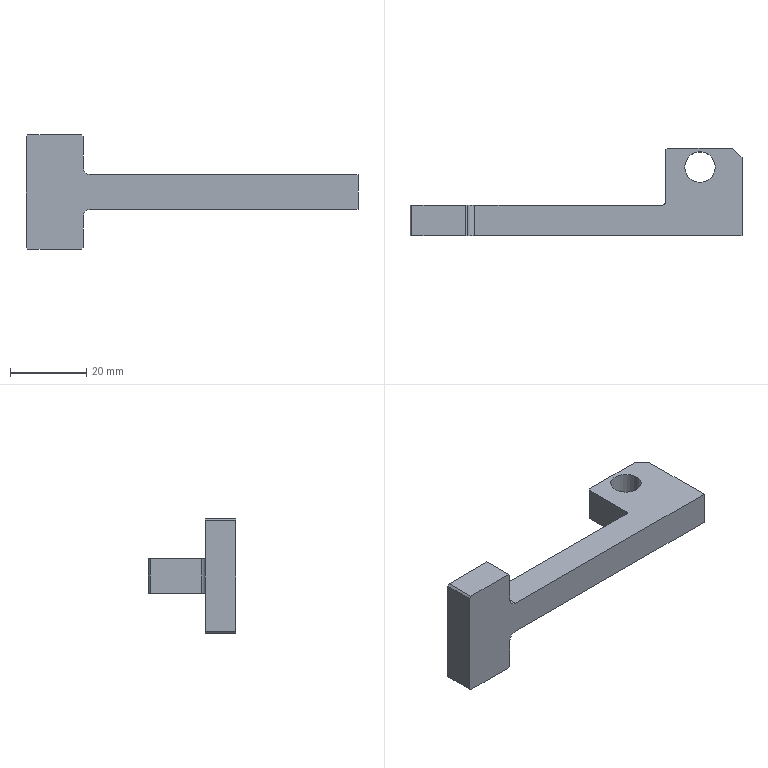Part | SolidWorks | features Chamfer 2, Fillet 2, ICE 2, Cut 1, Extrusion 1, MoveFace 1 | 1 solid | 23 faces | box 87 x 23 x 30 mm | volume 11014 mm3 | plane 18 | cylinder 5 | commonest cylinder face diameters 4 x2 8 x2 2 x1
STEP:
#1=CARTESIAN_POINT('',(80.,18.,9.));
#2=VERTEX_POINT('',#1);
#3=CARTESIAN_POINT('',(72.,18.,9.));
#4=VERTEX_POINT('',#3);
#5=CARTESIAN_POINT('',(76.,18.,9.));
#6=DIRECTION('',(0.,0.,-1.));
#7=DIRECTION('',(-1.,0.,0.));
#8=AXIS2_PLACEMENT_3D('',#5,#6,#7);
#9=CIRCLE('',#8,4.);
#10=EDGE_CURVE('',#2,#4,#9,.T.);
#11=ORIENTED_EDGE('',*,*,#10,.F.);
#12=CARTESIAN_POINT('',(80.,18.,0.));
#13=VERTEX_POINT('',#12);
#14=CARTESIAN_POINT('',(80.,18.,9.));
#15=DIRECTION('',(0.,0.,-1.));
#16=VECTOR('',#15,1000.);
#17=LINE('',#14,#16);
#18=EDGE_CURVE('',#2,#13,#17,.T.);
#19=ORIENTED_EDGE('',*,*,#18,.T.);
#20=CARTESIAN_POINT('',(72.,18.,0.));
#21=VERTEX_POINT('',#20);
#22=CARTESIAN_POINT('',(76.,18.,0.));
#23=DIRECTION('',(0.,0.,-1.));
#24=DIRECTION('',(-1.,0.,0.));
#25=AXIS2_PLACEMENT_3D('',#22,#23,#24);
#26=CIRCLE('',#25,4.);
#27=EDGE_CURVE('',#13,#21,#26,.T.);
#28=ORIENTED_EDGE('',*,*,#27,.T.);
#29=CARTESIAN_POINT('',(72.,18.,9.));
#30=DIRECTION('',(0.,0.,-1.));
#31=VECTOR('',#30,1000.);
#32=LINE('',#29,#31);
#33=EDGE_CURVE('',#4,#21,#32,.T.);
#34=ORIENTED_EDGE('',*,*,#33,.F.);
#35=EDGE_LOOP('',(#11,#19,#28,#34));
#36=FACE_OUTER_BOUND('',#35,.T.);
#37=CARTESIAN_POINT('',(76.,18.,9.));
#38=DIRECTION('',(0.,0.,-1.));
#39=DIRECTION('',(-1.,0.,0.));
#40=AXIS2_PLACEMENT_3D('',#37,#38,#39);
#41=CYLINDRICAL_SURFACE('',#40,4.);
#42=ADVANCED_FACE('',(#36),#41,.F.);
#43=CARTESIAN_POINT('',(0.,0.,-10.));
#44=VERTEX_POINT('',#43);
#45=CARTESIAN_POINT('',(0.,0.,19.));
#46=VERTEX_POINT('',#45);
#47=CARTESIAN_POINT('',(0.,0.,0.));
#48=DIRECTION('',(0.,0.,1.));
#49=VECTOR('',#48,1000.);
#50=LINE('',#47,#49);
#51=EDGE_CURVE('',#44,#46,#50,.T.);
#52=ORIENTED_EDGE('',*,*,#51,.T.);
#53=CARTESIAN_POINT('',(0.,8.,19.));
#54=VERTEX_POINT('',#53);
#55=CARTESIAN_POINT('',(0.,8.,19.));
#56=DIRECTION('',(0.,1.,0.));
#57=VECTOR('',#56,1000.);
#58=LINE('',#55,#57);
#59=EDGE_CURVE('',#46,#54,#58,.T.);
#60=ORIENTED_EDGE('',*,*,#59,.T.);
#61=CARTESIAN_POINT('',(0.,8.,-10.));
#62=VERTEX_POINT('',#61);
#63=CARTESIAN_POINT('',(0.,8.,0.));
#64=DIRECTION('',(0.,0.,1.));
#65=VECTOR('',#64,1000.);
#66=LINE('',#63,#65);
#67=EDGE_CURVE('',#62,#54,#66,.T.);
#68=ORIENTED_EDGE('',*,*,#67,.F.);
#69=CARTESIAN_POINT('',(0.,0.,-10.));
#70=DIRECTION('',(0.,-1.,0.));
#71=VECTOR('',#70,1000.);
#72=LINE('',#69,#71);
#73=EDGE_CURVE('',#62,#44,#72,.T.);
#74=ORIENTED_EDGE('',*,*,#73,.T.);
#75=EDGE_LOOP('',(#52,#60,#68,#74));
#76=FACE_OUTER_BOUND('',#75,.T.);
#77=CARTESIAN_POINT('',(0.,8.,0.));
#78=DIRECTION('',(1.,0.,0.));
#79=DIRECTION('',(0.,0.,-1.));
#80=AXIS2_PLACEMENT_3D('',#77,#78,#79);
#81=PLANE('',#80);
#82=ADVANCED_FACE('',(#76),#81,.F.);
#83=CARTESIAN_POINT('',(76.,18.,9.));
#84=DIRECTION('',(0.,0.,-1.));
#85=DIRECTION('',(-1.,0.,0.));
#86=AXIS2_PLACEMENT_3D('',#83,#84,#85);
#87=CIRCLE('',#86,4.);
#88=EDGE_CURVE('',#4,#2,#87,.T.);
#89=ORIENTED_EDGE('',*,*,#88,.T.);
#90=ORIENTED_EDGE('',*,*,#10,.T.);
#91=EDGE_LOOP('',(#89,#90));
#92=FACE_BOUND('',#91,.T.);
#93=CARTESIAN_POINT('',(17.,8.,9.));
#94=VERTEX_POINT('',#93);
#95=CARTESIAN_POINT('',(66.,8.,9.));
#96=VERTEX_POINT('',#95);
#97=CARTESIAN_POINT('',(0.,8.,9.));
#98=DIRECTION('',(1.,0.,0.));
#99=VECTOR('',#98,1000.);
#100=LINE('',#97,#99);
#101=EDGE_CURVE('',#94,#96,#100,.T.);
#102=ORIENTED_EDGE('',*,*,#101,.F.);
#103=CARTESIAN_POINT('',(17.,0.,9.));
#104=VERTEX_POINT('',#103);
#105=CARTESIAN_POINT('',(17.,8.,9.));
#106=DIRECTION('',(0.,-1.,0.));
#107=VECTOR('',#106,1000.);
#108=LINE('',#105,#107);
#109=EDGE_CURVE('',#94,#104,#108,.T.);
#110=ORIENTED_EDGE('',*,*,#109,.T.);
#111=CARTESIAN_POINT('',(87.,0.,9.));
#112=VERTEX_POINT('',#111);
#113=CARTESIAN_POINT('',(0.,0.,9.));
#114=DIRECTION('',(1.,0.,0.));
#115=VECTOR('',#114,1000.);
#116=LINE('',#113,#115);
#117=EDGE_CURVE('',#104,#112,#116,.T.);
#118=ORIENTED_EDGE('',*,*,#117,.T.);
#119=CARTESIAN_POINT('',(87.,20.5,9.));
#120=VERTEX_POINT('',#119);
#121=CARTESIAN_POINT('',(87.,8.,9.));
#122=DIRECTION('',(0.,-1.,0.));
#123=VECTOR('',#122,1000.);
#124=LINE('',#121,#123);
#125=EDGE_CURVE('',#120,#112,#124,.T.);
#126=ORIENTED_EDGE('',*,*,#125,.F.);
#127=CARTESIAN_POINT('',(84.5,23.,9.));
#128=VERTEX_POINT('',#127);
#129=CARTESIAN_POINT('',(84.5,23.,9.));
#130=DIRECTION('',(-0.7071,0.7071,0.));
#131=VECTOR('',#130,1000.);
#132=LINE('',#129,#131);
#133=EDGE_CURVE('',#120,#128,#132,.T.);
#134=ORIENTED_EDGE('',*,*,#133,.T.);
#135=CARTESIAN_POINT('',(67.5,23.,9.));
#136=VERTEX_POINT('',#135);
#137=CARTESIAN_POINT('',(85.,23.,9.));
#138=DIRECTION('',(1.,0.,0.));
#139=VECTOR('',#138,1000.);
#140=LINE('',#137,#139);
#141=EDGE_CURVE('',#136,#128,#140,.T.);
#142=ORIENTED_EDGE('',*,*,#141,.F.);
#143=CARTESIAN_POINT('',(67.,22.5,9.));
#144=VERTEX_POINT('',#143);
#145=CARTESIAN_POINT('',(67.5,23.,9.));
#146=DIRECTION('',(-0.7071,-0.7071,0.));
#147=VECTOR('',#146,1000.);
#148=LINE('',#145,#147);
#149=EDGE_CURVE('',#136,#144,#148,.T.);
#150=ORIENTED_EDGE('',*,*,#149,.T.);
#151=CARTESIAN_POINT('',(67.,9.,9.));
#152=VERTEX_POINT('',#151);
#153=CARTESIAN_POINT('',(67.,23.,9.));
#154=DIRECTION('',(0.,-1.,0.));
#155=VECTOR('',#154,1000.);
#156=LINE('',#153,#155);
#157=EDGE_CURVE('',#144,#152,#156,.T.);
#158=ORIENTED_EDGE('',*,*,#157,.T.);
#159=CARTESIAN_POINT('',(66.,9.,9.));
#160=DIRECTION('',(0.,0.,-1.));
#161=DIRECTION('',(-1.,0.,0.));
#162=AXIS2_PLACEMENT_3D('',#159,#160,#161);
#163=CIRCLE('',#162,1.);
#164=EDGE_CURVE('',#152,#96,#163,.T.);
#165=ORIENTED_EDGE('',*,*,#164,.T.);
#166=EDGE_LOOP('',(#102,#110,#118,#126,#134,#142,#150,#158,#165));
#167=FACE_OUTER_BOUND('',#166,.T.);
#168=CARTESIAN_POINT('',(0.,8.,9.));
#169=DIRECTION('',(0.,0.,-1.));
#170=DIRECTION('',(-1.,0.,0.));
#171=AXIS2_PLACEMENT_3D('',#168,#169,#170);
#172=PLANE('',#171);
#173=ADVANCED_FACE('',(#92,#167),#172,.F.);
#174=CARTESIAN_POINT('',(87.,20.5,0.));
#175=VERTEX_POINT('',#174);
#176=CARTESIAN_POINT('',(87.,0.,0.));
#177=VERTEX_POINT('',#176);
#178=CARTESIAN_POINT('',(87.,8.,0.));
#179=DIRECTION('',(0.,-1.,0.));
#180=VECTOR('',#179,1000.);
#181=LINE('',#178,#180);
#182=EDGE_CURVE('',#175,#177,#181,.T.);
#183=ORIENTED_EDGE('',*,*,#182,.F.);
#184=CARTESIAN_POINT('',(87.,20.5,0.));
#185=DIRECTION('',(0.,0.,1.));
#186=VECTOR('',#185,1000.);
#187=LINE('',#184,#186);
#188=EDGE_CURVE('',#175,#120,#187,.T.);
#189=ORIENTED_EDGE('',*,*,#188,.T.);
#190=ORIENTED_EDGE('',*,*,#125,.T.);
#191=CARTESIAN_POINT('',(87.,0.,0.));
#192=DIRECTION('',(0.,0.,-1.));
#193=VECTOR('',#192,1000.);
#194=LINE('',#191,#193);
#195=EDGE_CURVE('',#112,#177,#194,.T.);
#196=ORIENTED_EDGE('',*,*,#195,.T.);
#197=EDGE_LOOP('',(#183,#189,#190,#196));
#198=FACE_OUTER_BOUND('',#197,.T.);
#199=CARTESIAN_POINT('',(87.,8.,0.));
#200=DIRECTION('',(-1.,0.,0.));
#201=DIRECTION('',(0.,0.,1.));
#202=AXIS2_PLACEMENT_3D('',#199,#200,#201);
#203=PLANE('',#202);
#204=ADVANCED_FACE('',(#198),#203,.F.);
#205=CARTESIAN_POINT('',(76.,18.,0.));
#206=DIRECTION('',(0.,0.,-1.));
#207=DIRECTION('',(-1.,0.,0.));
#208=AXIS2_PLACEMENT_3D('',#205,#206,#207);
#209=CIRCLE('',#208,4.);
#210=EDGE_CURVE('',#21,#13,#209,.T.);
#211=ORIENTED_EDGE('',*,*,#210,.F.);
#212=ORIENTED_EDGE('',*,*,#27,.F.);
#213=EDGE_LOOP('',(#211,#212));
#214=FACE_BOUND('',#213,.T.);
#215=CARTESIAN_POINT('',(17.,0.,0.));
#216=VERTEX_POINT('',#215);
#217=CARTESIAN_POINT('',(0.,0.,0.));
#218=DIRECTION('',(-1.,0.,0.));
#219=VECTOR('',#218,1000.);
#220=LINE('',#217,#219);
#221=EDGE_CURVE('',#177,#216,#220,.T.);
#222=ORIENTED_EDGE('',*,*,#221,.T.);
#223=CARTESIAN_POINT('',(17.,8.,0.));
#224=VERTEX_POINT('',#223);
#225=CARTESIAN_POINT('',(17.,8.,0.));
#226=DIRECTION('',(0.,1.,0.));
#227=VECTOR('',#226,1000.);
#228=LINE('',#225,#227);
#229=EDGE_CURVE('',#216,#224,#228,.T.);
#230=ORIENTED_EDGE('',*,*,#229,.T.);
#231=CARTESIAN_POINT('',(66.,8.,0.));
#232=VERTEX_POINT('',#231);
#233=CARTESIAN_POINT('',(0.,8.,0.));
#234=DIRECTION('',(-1.,0.,0.));
#235=VECTOR('',#234,1000.);
#236=LINE('',#233,#235);
#237=EDGE_CURVE('',#232,#224,#236,.T.);
#238=ORIENTED_EDGE('',*,*,#237,.F.);
#239=CARTESIAN_POINT('',(67.,9.,0.));
#240=VERTEX_POINT('',#239);
#241=CARTESIAN_POINT('',(66.,9.,0.));
#242=DIRECTION('',(0.,0.,1.));
#243=DIRECTION('',(1.,0.,0.));
#244=AXIS2_PLACEMENT_3D('',#241,#242,#243);
#245=CIRCLE('',#244,1.);
#246=EDGE_CURVE('',#232,#240,#245,.T.);
#247=ORIENTED_EDGE('',*,*,#246,.T.);
#248=CARTESIAN_POINT('',(67.,22.5,0.));
#249=VERTEX_POINT('',#248);
#250=CARTESIAN_POINT('',(67.,23.,0.));
#251=DIRECTION('',(0.,-1.,0.));
#252=VECTOR('',#251,1000.);
#253=LINE('',#250,#252);
#254=EDGE_CURVE('',#249,#240,#253,.T.);
#255=ORIENTED_EDGE('',*,*,#254,.F.);
#256=CARTESIAN_POINT('',(67.5,23.,0.));
#257=VERTEX_POINT('',#256);
#258=CARTESIAN_POINT('',(67.5,23.,0.));
#259=DIRECTION('',(0.7071,0.7071,0.));
#260=VECTOR('',#259,1000.);
#261=LINE('',#258,#260);
#262=EDGE_CURVE('',#249,#257,#261,.T.);
#263=ORIENTED_EDGE('',*,*,#262,.T.);
#264=CARTESIAN_POINT('',(84.5,23.,0.));
#265=VERTEX_POINT('',#264);
#266=CARTESIAN_POINT('',(85.,23.,0.));
#267=DIRECTION('',(-1.,0.,0.));
#268=VECTOR('',#267,1000.);
#269=LINE('',#266,#268);
#270=EDGE_CURVE('',#265,#257,#269,.T.);
#271=ORIENTED_EDGE('',*,*,#270,.F.);
#272=CARTESIAN_POINT('',(84.5,23.,0.));
#273=DIRECTION('',(0.7071,-0.7071,0.));
#274=VECTOR('',#273,1000.);
#275=LINE('',#272,#274);
#276=EDGE_CURVE('',#265,#175,#275,.T.);
#277=ORIENTED_EDGE('',*,*,#276,.T.);
#278=ORIENTED_EDGE('',*,*,#182,.T.);
#279=EDGE_LOOP('',(#222,#230,#238,#247,#255,#263,#271,#277,#278));
#280=FACE_OUTER_BOUND('',#279,.T.);
#281=CARTESIAN_POINT('',(0.,8.,0.));
#282=DIRECTION('',(0.,0.,1.));
#283=DIRECTION('',(1.,0.,0.));
#284=AXIS2_PLACEMENT_3D('',#281,#282,#283);
#285=PLANE('',#284);
#286=ADVANCED_FACE('',(#214,#280),#285,.F.);
#287=ORIENTED_EDGE('',*,*,#101,.T.);
#288=CARTESIAN_POINT('',(66.,8.,0.));
#289=DIRECTION('',(0.,0.,-1.));
#290=VECTOR('',#289,1000.);
#291=LINE('',#288,#290);
#292=EDGE_CURVE('',#96,#232,#291,.T.);
#293=ORIENTED_EDGE('',*,*,#292,.T.);
#294=ORIENTED_EDGE('',*,*,#237,.T.);
#295=CARTESIAN_POINT('',(15.,8.,-2.));
#296=VERTEX_POINT('',#295);
#297=CARTESIAN_POINT('',(17.,8.,-2.));
#298=DIRECTION('',(0.,-1.,0.));
#299=DIRECTION('',(0.,0.,1.));
#300=AXIS2_PLACEMENT_3D('',#297,#298,#299);
#301=CIRCLE('',#300,2.);
#302=EDGE_CURVE('',#224,#296,#301,.T.);
#303=ORIENTED_EDGE('',*,*,#302,.T.);
#304=CARTESIAN_POINT('',(15.,8.,-10.));
#305=VERTEX_POINT('',#304);
#306=CARTESIAN_POINT('',(15.,8.,-10.5));
#307=DIRECTION('',(0.,0.,1.));
#308=VECTOR('',#307,1000.);
#309=LINE('',#306,#308);
#310=EDGE_CURVE('',#305,#296,#309,.T.);
#311=ORIENTED_EDGE('',*,*,#310,.F.);
#312=CARTESIAN_POINT('',(14.5,8.,-10.5));
#313=VERTEX_POINT('',#312);
#314=CARTESIAN_POINT('',(12.5,8.,-12.5));
#315=DIRECTION('',(-0.7071,0.,-0.7071));
#316=VECTOR('',#315,1000.);
#317=LINE('',#314,#316);
#318=EDGE_CURVE('',#305,#313,#317,.T.);
#319=ORIENTED_EDGE('',*,*,#318,.T.);
#320=CARTESIAN_POINT('',(0.5,8.,-10.5));
#321=VERTEX_POINT('',#320);
#322=CARTESIAN_POINT('',(15.,8.,-10.5));
#323=DIRECTION('',(1.,0.,0.));
#324=VECTOR('',#323,1000.);
#325=LINE('',#322,#324);
#326=EDGE_CURVE('',#321,#313,#325,.T.);
#327=ORIENTED_EDGE('',*,*,#326,.F.);
#328=CARTESIAN_POINT('',(-5.,8.,-5.));
#329=DIRECTION('',(-0.7071,0.,0.7071));
#330=VECTOR('',#329,1000.);
#331=LINE('',#328,#330);
#332=EDGE_CURVE('',#321,#62,#331,.T.);
#333=ORIENTED_EDGE('',*,*,#332,.T.);
#334=ORIENTED_EDGE('',*,*,#67,.T.);
#335=CARTESIAN_POINT('',(0.5,8.,19.5));
#336=VERTEX_POINT('',#335);
#337=CARTESIAN_POINT('',(-9.5,8.,9.5));
#338=DIRECTION('',(0.7071,0.,0.7071));
#339=VECTOR('',#338,1000.);
#340=LINE('',#337,#339);
#341=EDGE_CURVE('',#54,#336,#340,.T.);
#342=ORIENTED_EDGE('',*,*,#341,.T.);
#343=CARTESIAN_POINT('',(14.5,8.,19.5));
#344=VERTEX_POINT('',#343);
#345=CARTESIAN_POINT('',(15.,8.,19.5));
#346=DIRECTION('',(-1.,0.,0.));
#347=VECTOR('',#346,1000.);
#348=LINE('',#345,#347);
#349=EDGE_CURVE('',#344,#336,#348,.T.);
#350=ORIENTED_EDGE('',*,*,#349,.F.);
#351=CARTESIAN_POINT('',(15.,8.,19.));
#352=VERTEX_POINT('',#351);
#353=CARTESIAN_POINT('',(17.,8.,17.));
#354=DIRECTION('',(0.7071,0.,-0.7071));
#355=VECTOR('',#354,1000.);
#356=LINE('',#353,#355);
#357=EDGE_CURVE('',#344,#352,#356,.T.);
#358=ORIENTED_EDGE('',*,*,#357,.T.);
#359=CARTESIAN_POINT('',(15.,8.,11.));
#360=VERTEX_POINT('',#359);
#361=CARTESIAN_POINT('',(15.,8.,-10.5));
#362=DIRECTION('',(0.,0.,1.));
#363=VECTOR('',#362,1000.);
#364=LINE('',#361,#363);
#365=EDGE_CURVE('',#360,#352,#364,.T.);
#366=ORIENTED_EDGE('',*,*,#365,.F.);
#367=CARTESIAN_POINT('',(17.,8.,11.));
#368=DIRECTION('',(0.,-1.,0.));
#369=DIRECTION('',(0.,0.,1.));
#370=AXIS2_PLACEMENT_3D('',#367,#368,#369);
#371=CIRCLE('',#370,2.);
#372=EDGE_CURVE('',#360,#94,#371,.T.);
#373=ORIENTED_EDGE('',*,*,#372,.T.);
#374=EDGE_LOOP('',(#287,#293,#294,#303,#311,#319,#327,#333,#334,#342,#350,#358,#366,#373));
#375=FACE_OUTER_BOUND('',#374,.T.);
#376=CARTESIAN_POINT('',(0.,8.,0.));
#377=DIRECTION('',(0.,1.,0.));
#378=DIRECTION('',(0.,0.,1.));
#379=AXIS2_PLACEMENT_3D('',#376,#377,#378);
#380=PLANE('',#379);
#381=ADVANCED_FACE('',(#375),#380,.T.);
#382=CARTESIAN_POINT('',(14.5,0.,19.5));
#383=VERTEX_POINT('',#382);
#384=CARTESIAN_POINT('',(0.5,0.,19.5));
#385=VERTEX_POINT('',#384);
#386=CARTESIAN_POINT('',(15.,0.,19.5));
#387=DIRECTION('',(-1.,0.,0.));
#388=VECTOR('',#387,1000.);
#389=LINE('',#386,#388);
#390=EDGE_CURVE('',#383,#385,#389,.T.);
#391=ORIENTED_EDGE('',*,*,#390,.T.);
#392=CARTESIAN_POINT('',(0.5,0.,19.5));
#393=DIRECTION('',(-0.7071,0.,-0.7071));
#394=VECTOR('',#393,1000.);
#395=LINE('',#392,#394);
#396=EDGE_CURVE('',#385,#46,#395,.T.);
#397=ORIENTED_EDGE('',*,*,#396,.T.);
#398=ORIENTED_EDGE('',*,*,#51,.F.);
#399=CARTESIAN_POINT('',(0.5,0.,-10.5));
#400=VERTEX_POINT('',#399);
#401=CARTESIAN_POINT('',(0.,0.,-10.));
#402=DIRECTION('',(0.7071,0.,-0.7071));
#403=VECTOR('',#402,1000.);
#404=LINE('',#401,#403);
#405=EDGE_CURVE('',#44,#400,#404,.T.);
#406=ORIENTED_EDGE('',*,*,#405,.T.);
#407=CARTESIAN_POINT('',(14.5,0.,-10.5));
#408=VERTEX_POINT('',#407);
#409=CARTESIAN_POINT('',(15.,0.,-10.5));
#410=DIRECTION('',(1.,0.,0.));
#411=VECTOR('',#410,1000.);
#412=LINE('',#409,#411);
#413=EDGE_CURVE('',#400,#408,#412,.T.);
#414=ORIENTED_EDGE('',*,*,#413,.T.);
#415=CARTESIAN_POINT('',(15.,0.,-10.));
#416=VERTEX_POINT('',#415);
#417=CARTESIAN_POINT('',(14.5,0.,-10.5));
#418=DIRECTION('',(0.7071,0.,0.7071));
#419=VECTOR('',#418,1000.);
#420=LINE('',#417,#419);
#421=EDGE_CURVE('',#408,#416,#420,.T.);
#422=ORIENTED_EDGE('',*,*,#421,.T.);
#423=CARTESIAN_POINT('',(15.,0.,-2.));
#424=VERTEX_POINT('',#423);
#425=CARTESIAN_POINT('',(15.,0.,-10.5));
#426=DIRECTION('',(0.,0.,1.));
#427=VECTOR('',#426,1000.);
#428=LINE('',#425,#427);
#429=EDGE_CURVE('',#416,#424,#428,.T.);
#430=ORIENTED_EDGE('',*,*,#429,.T.);
#431=CARTESIAN_POINT('',(17.,0.,-2.));
#432=DIRECTION('',(0.,1.,0.));
#433=DIRECTION('',(0.,0.,1.));
#434=AXIS2_PLACEMENT_3D('',#431,#432,#433);
#435=CIRCLE('',#434,2.);
#436=EDGE_CURVE('',#424,#216,#435,.T.);
#437=ORIENTED_EDGE('',*,*,#436,.T.);
#438=ORIENTED_EDGE('',*,*,#221,.F.);
#439=ORIENTED_EDGE('',*,*,#195,.F.);
#440=ORIENTED_EDGE('',*,*,#117,.F.);
#441=CARTESIAN_POINT('',(15.,0.,11.));
#442=VERTEX_POINT('',#441);
#443=CARTESIAN_POINT('',(17.,0.,11.));
#444=DIRECTION('',(0.,1.,0.));
#445=DIRECTION('',(0.,0.,1.));
#446=AXIS2_PLACEMENT_3D('',#443,#444,#445);
#447=CIRCLE('',#446,2.);
#448=EDGE_CURVE('',#104,#442,#447,.T.);
#449=ORIENTED_EDGE('',*,*,#448,.T.);
#450=CARTESIAN_POINT('',(15.,0.,19.));
#451=VERTEX_POINT('',#450);
#452=CARTESIAN_POINT('',(15.,0.,-10.5));
#453=DIRECTION('',(0.,0.,1.));
#454=VECTOR('',#453,1000.);
#455=LINE('',#452,#454);
#456=EDGE_CURVE('',#442,#451,#455,.T.);
#457=ORIENTED_EDGE('',*,*,#456,.T.);
#458=CARTESIAN_POINT('',(15.,0.,19.));
#459=DIRECTION('',(-0.7071,0.,0.7071));
#460=VECTOR('',#459,1000.);
#461=LINE('',#458,#460);
#462=EDGE_CURVE('',#451,#383,#461,.T.);
#463=ORIENTED_EDGE('',*,*,#462,.T.);
#464=EDGE_LOOP('',(#391,#397,#398,#406,#414,#422,#430,#437,#438,#439,#440,#449,#457,#463));
#465=FACE_OUTER_BOUND('',#464,.T.);
#466=CARTESIAN_POINT('',(0.,0.,0.));
#467=DIRECTION('',(0.,1.,0.));
#468=DIRECTION('',(0.,0.,1.));
#469=AXIS2_PLACEMENT_3D('',#466,#467,#468);
#470=PLANE('',#469);
#471=ADVANCED_FACE('',(#465),#470,.F.);
#472=ORIENTED_EDGE('',*,*,#254,.T.);
#473=CARTESIAN_POINT('',(67.,9.,0.));
#474=DIRECTION('',(0.,0.,1.));
#475=VECTOR('',#474,1000.);
#476=LINE('',#473,#475);
#477=EDGE_CURVE('',#240,#152,#476,.T.);
#478=ORIENTED_EDGE('',*,*,#477,.T.);
#479=ORIENTED_EDGE('',*,*,#157,.F.);
#480=CARTESIAN_POINT('',(67.,22.5,0.));
#481=DIRECTION('',(0.,0.,-1.));
#482=VECTOR('',#481,1000.);
#483=LINE('',#480,#482);
#484=EDGE_CURVE('',#144,#249,#483,.T.);
#485=ORIENTED_EDGE('',*,*,#484,.T.);
#486=EDGE_LOOP('',(#472,#478,#479,#485));
#487=FACE_OUTER_BOUND('',#486,.T.);
#488=CARTESIAN_POINT('',(67.,23.,0.));
#489=DIRECTION('',(1.,0.,0.));
#490=DIRECTION('',(0.,0.,-1.));
#491=AXIS2_PLACEMENT_3D('',#488,#489,#490);
#492=PLANE('',#491);
#493=ADVANCED_FACE('',(#487),#492,.F.);
#494=ORIENTED_EDGE('',*,*,#141,.T.);
#495=CARTESIAN_POINT('',(84.5,23.,0.));
#496=DIRECTION('',(0.,0.,-1.));
#497=VECTOR('',#496,1000.);
#498=LINE('',#495,#497);
#499=EDGE_CURVE('',#128,#265,#498,.T.);
#500=ORIENTED_EDGE('',*,*,#499,.T.);
#501=ORIENTED_EDGE('',*,*,#270,.T.);
#502=CARTESIAN_POINT('',(67.5,23.,0.));
#503=DIRECTION('',(0.,0.,1.));
#504=VECTOR('',#503,1000.);
#505=LINE('',#502,#504);
#506=EDGE_CURVE('',#257,#136,#505,.T.);
#507=ORIENTED_EDGE('',*,*,#506,.T.);
#508=EDGE_LOOP('',(#494,#500,#501,#507));
#509=FACE_OUTER_BOUND('',#508,.T.);
#510=CARTESIAN_POINT('',(0.,23.,0.));
#511=DIRECTION('',(0.,-1.,0.));
#512=DIRECTION('',(0.,0.,-1.));
#513=AXIS2_PLACEMENT_3D('',#510,#511,#512);
#514=PLANE('',#513);
#515=ADVANCED_FACE('',(#509),#514,.F.);
#516=ORIENTED_EDGE('',*,*,#18,.F.);
#517=ORIENTED_EDGE('',*,*,#88,.F.);
#518=ORIENTED_EDGE('',*,*,#33,.T.);
#519=ORIENTED_EDGE('',*,*,#210,.T.);
#520=EDGE_LOOP('',(#516,#517,#518,#519));
#521=FACE_OUTER_BOUND('',#520,.T.);
#522=CARTESIAN_POINT('',(76.,18.,9.));
#523=DIRECTION('',(0.,0.,-1.));
#524=DIRECTION('',(-1.,0.,0.));
#525=AXIS2_PLACEMENT_3D('',#522,#523,#524);
#526=CYLINDRICAL_SURFACE('',#525,4.);
#527=ADVANCED_FACE('',(#521),#526,.F.);
#528=ORIENTED_EDGE('',*,*,#133,.F.);
#529=ORIENTED_EDGE('',*,*,#188,.F.);
#530=ORIENTED_EDGE('',*,*,#276,.F.);
#531=ORIENTED_EDGE('',*,*,#499,.F.);
#532=EDGE_LOOP('',(#528,#529,#530,#531));
#533=FACE_OUTER_BOUND('',#532,.T.);
#534=CARTESIAN_POINT('',(84.5,23.,0.));
#535=DIRECTION('',(-0.7071,-0.7071,0.));
#536=DIRECTION('',(0.,0.,-1.));
#537=AXIS2_PLACEMENT_3D('',#534,#535,#536);
#538=PLANE('',#537);
#539=ADVANCED_FACE('',(#533),#538,.F.);
#540=ORIENTED_EDGE('',*,*,#262,.F.);
#541=ORIENTED_EDGE('',*,*,#484,.F.);
#542=ORIENTED_EDGE('',*,*,#149,.F.);
#543=ORIENTED_EDGE('',*,*,#506,.F.);
#544=EDGE_LOOP('',(#540,#541,#542,#543));
#545=FACE_OUTER_BOUND('',#544,.T.);
#546=CARTESIAN_POINT('',(67.5,23.,0.));
#547=DIRECTION('',(0.7071,-0.7071,0.));
#548=DIRECTION('',(0.,0.,1.));
#549=AXIS2_PLACEMENT_3D('',#546,#547,#548);
#550=PLANE('',#549);
#551=ADVANCED_FACE('',(#545),#550,.F.);
#552=ORIENTED_EDGE('',*,*,#413,.F.);
#553=CARTESIAN_POINT('',(0.5,8.,-10.5));
#554=DIRECTION('',(0.,1.,0.));
#555=VECTOR('',#554,1000.);
#556=LINE('',#553,#555);
#557=EDGE_CURVE('',#400,#321,#556,.T.);
#558=ORIENTED_EDGE('',*,*,#557,.T.);
#559=ORIENTED_EDGE('',*,*,#326,.T.);
#560=CARTESIAN_POINT('',(14.5,41.541,-10.5));
#561=DIRECTION('',(0.,-1.,0.));
#562=VECTOR('',#561,1000.);
#563=LINE('',#560,#562);
#564=EDGE_CURVE('',#313,#408,#563,.T.);
#565=ORIENTED_EDGE('',*,*,#564,.T.);
#566=EDGE_LOOP('',(#552,#558,#559,#565));
#567=FACE_OUTER_BOUND('',#566,.T.);
#568=CARTESIAN_POINT('',(15.,41.541,-10.5));
#569=DIRECTION('',(0.,0.,-1.));
#570=DIRECTION('',(-1.,0.,0.));
#571=AXIS2_PLACEMENT_3D('',#568,#569,#570);
#572=PLANE('',#571);
#573=ADVANCED_FACE('',(#567),#572,.T.);
#574=ORIENTED_EDGE('',*,*,#429,.F.);
#575=CARTESIAN_POINT('',(15.,41.541,-10.));
#576=DIRECTION('',(0.,1.,0.));
#577=VECTOR('',#576,1000.);
#578=LINE('',#575,#577);
#579=EDGE_CURVE('',#416,#305,#578,.T.);
#580=ORIENTED_EDGE('',*,*,#579,.T.);
#581=ORIENTED_EDGE('',*,*,#310,.T.);
#582=CARTESIAN_POINT('',(15.,41.541,-2.));
#583=DIRECTION('',(0.,-1.,0.));
#584=VECTOR('',#583,1000.);
#585=LINE('',#582,#584);
#586=EDGE_CURVE('',#296,#424,#585,.T.);
#587=ORIENTED_EDGE('',*,*,#586,.T.);
#588=EDGE_LOOP('',(#574,#580,#581,#587));
#589=FACE_OUTER_BOUND('',#588,.T.);
#590=CARTESIAN_POINT('',(15.,41.541,-10.5));
#591=DIRECTION('',(1.,0.,0.));
#592=DIRECTION('',(0.,0.,-1.));
#593=AXIS2_PLACEMENT_3D('',#590,#591,#592);
#594=PLANE('',#593);
#595=ADVANCED_FACE('',(#589),#594,.T.);
#596=ORIENTED_EDGE('',*,*,#365,.T.);
#597=CARTESIAN_POINT('',(15.,41.541,19.));
#598=DIRECTION('',(0.,-1.,0.));
#599=VECTOR('',#598,1000.);
#600=LINE('',#597,#599);
#601=EDGE_CURVE('',#352,#451,#600,.T.);
#602=ORIENTED_EDGE('',*,*,#601,.T.);
#603=ORIENTED_EDGE('',*,*,#456,.F.);
#604=CARTESIAN_POINT('',(15.,41.541,11.));
#605=DIRECTION('',(0.,1.,0.));
#606=VECTOR('',#605,1000.);
#607=LINE('',#604,#606);
#608=EDGE_CURVE('',#442,#360,#607,.T.);
#609=ORIENTED_EDGE('',*,*,#608,.T.);
#610=EDGE_LOOP('',(#596,#602,#603,#609));
#611=FACE_OUTER_BOUND('',#610,.T.);
#612=CARTESIAN_POINT('',(15.,41.541,-10.5));
#613=DIRECTION('',(1.,0.,0.));
#614=DIRECTION('',(0.,0.,-1.));
#615=AXIS2_PLACEMENT_3D('',#612,#613,#614);
#616=PLANE('',#615);
#617=ADVANCED_FACE('',(#611),#616,.T.);
#618=ORIENTED_EDGE('',*,*,#349,.T.);
#619=CARTESIAN_POINT('',(0.5,0.,19.5));
#620=DIRECTION('',(0.,-1.,0.));
#621=VECTOR('',#620,1000.);
#622=LINE('',#619,#621);
#623=EDGE_CURVE('',#336,#385,#622,.T.);
#624=ORIENTED_EDGE('',*,*,#623,.T.);
#625=ORIENTED_EDGE('',*,*,#390,.F.);
#626=CARTESIAN_POINT('',(14.5,41.541,19.5));
#627=DIRECTION('',(0.,1.,0.));
#628=VECTOR('',#627,1000.);
#629=LINE('',#626,#628);
#630=EDGE_CURVE('',#383,#344,#629,.T.);
#631=ORIENTED_EDGE('',*,*,#630,.T.);
#632=EDGE_LOOP('',(#618,#624,#625,#631));
#633=FACE_OUTER_BOUND('',#632,.T.);
#634=CARTESIAN_POINT('',(15.,41.541,19.5));
#635=DIRECTION('',(0.,0.,1.));
#636=DIRECTION('',(1.,0.,0.));
#637=AXIS2_PLACEMENT_3D('',#634,#635,#636);
#638=PLANE('',#637);
#639=ADVANCED_FACE('',(#633),#638,.T.);
#640=ORIENTED_EDGE('',*,*,#436,.F.);
#641=ORIENTED_EDGE('',*,*,#586,.F.);
#642=ORIENTED_EDGE('',*,*,#302,.F.);
#643=ORIENTED_EDGE('',*,*,#229,.F.);
#644=EDGE_LOOP('',(#640,#641,#642,#643));
#645=FACE_OUTER_BOUND('',#644,.T.);
#646=CARTESIAN_POINT('',(17.,8.,-2.));
#647=DIRECTION('',(0.,1.,0.));
#648=DIRECTION('',(0.,0.,1.));
#649=AXIS2_PLACEMENT_3D('',#646,#647,#648);
#650=CYLINDRICAL_SURFACE('',#649,2.);
#651=ADVANCED_FACE('',(#645),#650,.F.);
#652=ORIENTED_EDGE('',*,*,#372,.F.);
#653=ORIENTED_EDGE('',*,*,#608,.F.);
#654=ORIENTED_EDGE('',*,*,#448,.F.);
#655=ORIENTED_EDGE('',*,*,#109,.F.);
#656=EDGE_LOOP('',(#652,#653,#654,#655));
#657=FACE_OUTER_BOUND('',#656,.T.);
#658=CARTESIAN_POINT('',(17.,8.,11.));
#659=DIRECTION('',(0.,-1.,0.));
#660=DIRECTION('',(0.,0.,-1.));
#661=AXIS2_PLACEMENT_3D('',#658,#659,#660);
#662=CYLINDRICAL_SURFACE('',#661,2.);
#663=ADVANCED_FACE('',(#657),#662,.F.);
#664=ORIENTED_EDGE('',*,*,#341,.F.);
#665=ORIENTED_EDGE('',*,*,#59,.F.);
#666=ORIENTED_EDGE('',*,*,#396,.F.);
#667=ORIENTED_EDGE('',*,*,#623,.F.);
#668=EDGE_LOOP('',(#664,#665,#666,#667));
#669=FACE_OUTER_BOUND('',#668,.T.);
#670=CARTESIAN_POINT('',(0.5,41.541,19.5));
#671=DIRECTION('',(-0.7071,0.,0.7071));
#672=DIRECTION('',(0.,1.,0.));
#673=AXIS2_PLACEMENT_3D('',#670,#671,#672);
#674=PLANE('',#673);
#675=ADVANCED_FACE('',(#669),#674,.T.);
#676=ORIENTED_EDGE('',*,*,#357,.F.);
#677=ORIENTED_EDGE('',*,*,#630,.F.);
#678=ORIENTED_EDGE('',*,*,#462,.F.);
#679=ORIENTED_EDGE('',*,*,#601,.F.);
#680=EDGE_LOOP('',(#676,#677,#678,#679));
#681=FACE_OUTER_BOUND('',#680,.T.);
#682=CARTESIAN_POINT('',(15.,41.541,19.));
#683=DIRECTION('',(-0.7071,0.,-0.7071));
#684=DIRECTION('',(0.,-1.,0.));
#685=AXIS2_PLACEMENT_3D('',#682,#683,#684);
#686=PLANE('',#685);
#687=ADVANCED_FACE('',(#681),#686,.F.);
#688=ORIENTED_EDGE('',*,*,#332,.F.);
#689=ORIENTED_EDGE('',*,*,#557,.F.);
#690=ORIENTED_EDGE('',*,*,#405,.F.);
#691=ORIENTED_EDGE('',*,*,#73,.F.);
#692=EDGE_LOOP('',(#688,#689,#690,#691));
#693=FACE_OUTER_BOUND('',#692,.T.);
#694=CARTESIAN_POINT('',(0.,8.,-10.));
#695=DIRECTION('',(-0.7071,0.,-0.7071));
#696=DIRECTION('',(0.,1.,0.));
#697=AXIS2_PLACEMENT_3D('',#694,#695,#696);
#698=PLANE('',#697);
#699=ADVANCED_FACE('',(#693),#698,.T.);
#700=ORIENTED_EDGE('',*,*,#318,.F.);
#701=ORIENTED_EDGE('',*,*,#579,.F.);
#702=ORIENTED_EDGE('',*,*,#421,.F.);
#703=ORIENTED_EDGE('',*,*,#564,.F.);
#704=EDGE_LOOP('',(#700,#701,#702,#703));
#705=FACE_OUTER_BOUND('',#704,.T.);
#706=CARTESIAN_POINT('',(14.5,41.541,-10.5));
#707=DIRECTION('',(-0.7071,0.,0.7071));
#708=DIRECTION('',(0.,-1.,0.));
#709=AXIS2_PLACEMENT_3D('',#706,#707,#708);
#710=PLANE('',#709);
#711=ADVANCED_FACE('',(#705),#710,.F.);
#712=ORIENTED_EDGE('',*,*,#246,.F.);
#713=ORIENTED_EDGE('',*,*,#292,.F.);
#714=ORIENTED_EDGE('',*,*,#164,.F.);
#715=ORIENTED_EDGE('',*,*,#477,.F.);
#716=EDGE_LOOP('',(#712,#713,#714,#715));
#717=FACE_OUTER_BOUND('',#716,.T.);
#718=CARTESIAN_POINT('',(66.,9.,0.));
#719=DIRECTION('',(0.,0.,1.));
#720=DIRECTION('',(1.,0.,0.));
#721=AXIS2_PLACEMENT_3D('',#718,#719,#720);
#722=CYLINDRICAL_SURFACE('',#721,1.);
#723=ADVANCED_FACE('',(#717),#722,.F.);
#724=CLOSED_SHELL('',(#42,#82,#173,#204,#286,#381,#471,#493,#515,#527,#539,#551,#573,#595,#617,#639,#651,#663,#675,#687,#699,#711,#723));
#725=MANIFOLD_SOLID_BREP('',#724);
#726=CARTESIAN_POINT('',(0.,0.,0.));
#727=DIRECTION('',(0.,0.,1.));
#728=DIRECTION('',(1.,0.,0.));
#729=AXIS2_PLACEMENT_3D('',#726,#727,#728);
#730=(LENGTH_UNIT()NAMED_UNIT(*)SI_UNIT(.MILLI.,.METRE.));
#731=UNCERTAINTY_MEASURE_WITH_UNIT(LENGTH_MEASURE(0.00001),#730,'','');
#732=(NAMED_UNIT(*)PLANE_ANGLE_UNIT()SI_UNIT($,.RADIAN.));
#733=(NAMED_UNIT(*)SI_UNIT($,.STERADIAN.)SOLID_ANGLE_UNIT());
#734=(GEOMETRIC_REPRESENTATION_CONTEXT(3)GLOBAL_UNCERTAINTY_ASSIGNED_CONTEXT((#731))GLOBAL_UNIT_ASSIGNED_CONTEXT((#730,#732,#733))REPRESENTATION_CONTEXT('',''));
#735=ADVANCED_BREP_SHAPE_REPRESENTATION('',(#725,#729),#734);